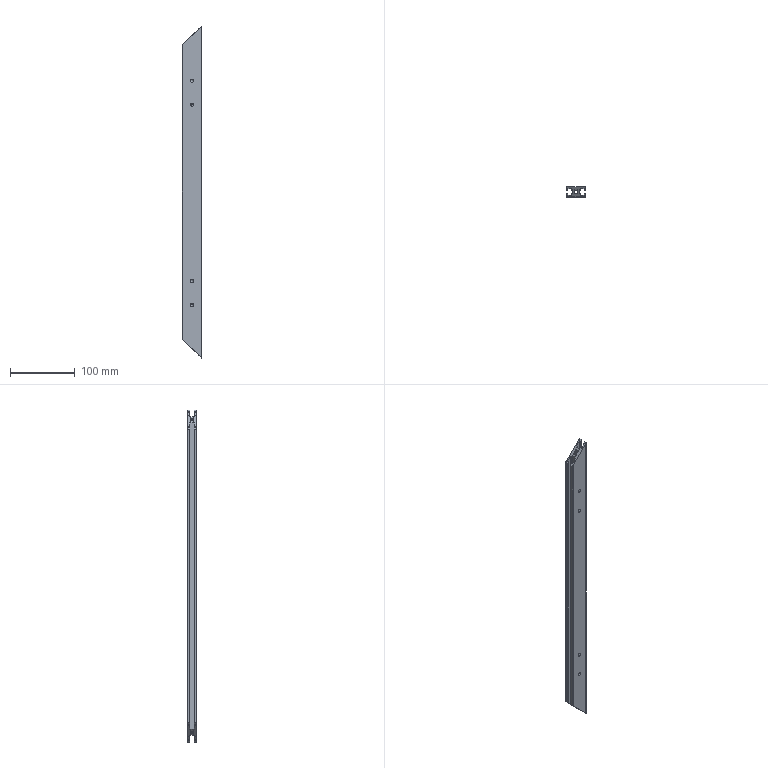Part | NX | features BREP 1 | 1 solid | 129 faces | box 30 x 15 x 512.1 mm | volume 115658 mm3 | cylinder 67 | plane 54 | cone 8 | commonest cylinder face diameters 5 x57 1 x6 2 x4